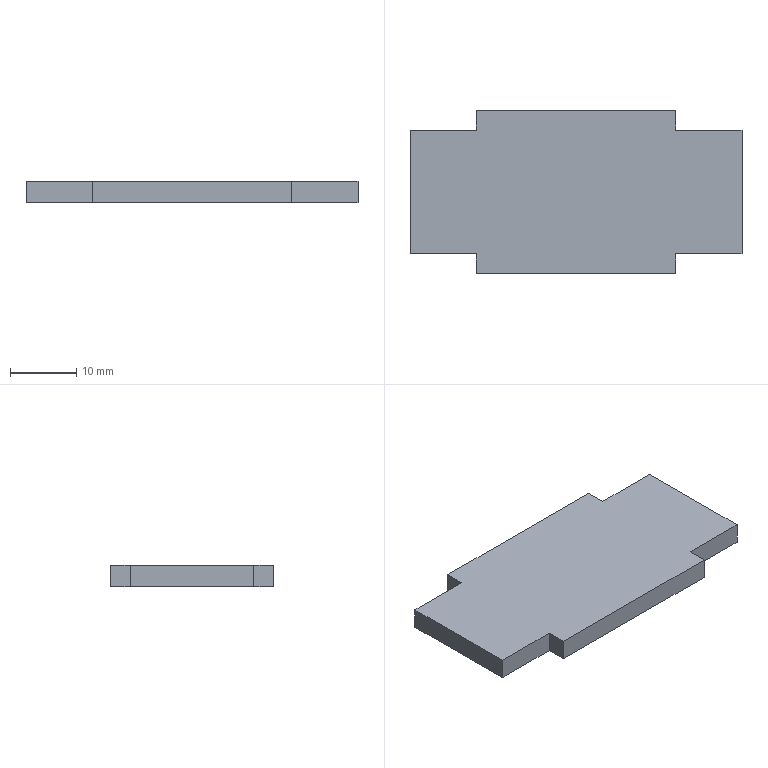Part | SolidWorks | features FlatPattern 1, SMBaseFlange 1, SheetMetal 1 | 1 solid | 14 faces | box 50 x 24.6 x 3.2 mm | volume 3552 mm3 | plane 14
STEP:
#1=CARTESIAN_POINT('',(95.,21.8,0.));
#2=VERTEX_POINT('',#1);
#3=CARTESIAN_POINT('',(95.,3.2,0.));
#4=VERTEX_POINT('',#3);
#5=CARTESIAN_POINT('',(95.,3.2,0.));
#6=DIRECTION('',(0.,-1.,0.));
#7=VECTOR('',#6,1000.);
#8=LINE('',#5,#7);
#9=EDGE_CURVE('',#2,#4,#8,.T.);
#10=ORIENTED_EDGE('',*,*,#9,.F.);
#11=CARTESIAN_POINT('',(95.,21.8,-3.2));
#12=VERTEX_POINT('',#11);
#13=CARTESIAN_POINT('',(95.,21.8,-3.2));
#14=DIRECTION('',(0.,0.,1.));
#15=VECTOR('',#14,1000.);
#16=LINE('',#13,#15);
#17=EDGE_CURVE('',#12,#2,#16,.T.);
#18=ORIENTED_EDGE('',*,*,#17,.F.);
#19=CARTESIAN_POINT('',(95.,3.2,-3.2));
#20=VERTEX_POINT('',#19);
#21=CARTESIAN_POINT('',(95.,3.2,-3.2));
#22=DIRECTION('',(0.,-1.,0.));
#23=VECTOR('',#22,1000.);
#24=LINE('',#21,#23);
#25=EDGE_CURVE('',#12,#20,#24,.T.);
#26=ORIENTED_EDGE('',*,*,#25,.T.);
#27=CARTESIAN_POINT('',(95.,3.2,-3.2));
#28=DIRECTION('',(0.,0.,1.));
#29=VECTOR('',#28,1000.);
#30=LINE('',#27,#29);
#31=EDGE_CURVE('',#20,#4,#30,.T.);
#32=ORIENTED_EDGE('',*,*,#31,.T.);
#33=EDGE_LOOP('',(#10,#18,#26,#32));
#34=FACE_OUTER_BOUND('',#33,.T.);
#35=CARTESIAN_POINT('',(95.,3.2,-3.2));
#36=DIRECTION('',(-1.,0.,0.));
#37=DIRECTION('',(0.,0.,1.));
#38=AXIS2_PLACEMENT_3D('',#35,#36,#37);
#39=PLANE('',#38);
#40=ADVANCED_FACE('',(#34),#39,.T.);
#41=CARTESIAN_POINT('',(105.,21.8,0.));
#42=VERTEX_POINT('',#41);
#43=CARTESIAN_POINT('',(95.,21.8,0.));
#44=DIRECTION('',(-1.,0.,0.));
#45=VECTOR('',#44,1000.);
#46=LINE('',#43,#45);
#47=EDGE_CURVE('',#42,#2,#46,.T.);
#48=ORIENTED_EDGE('',*,*,#47,.F.);
#49=CARTESIAN_POINT('',(105.,21.8,-3.2));
#50=VERTEX_POINT('',#49);
#51=CARTESIAN_POINT('',(105.,21.8,-3.2));
#52=DIRECTION('',(0.,0.,1.));
#53=VECTOR('',#52,1000.);
#54=LINE('',#51,#53);
#55=EDGE_CURVE('',#50,#42,#54,.T.);
#56=ORIENTED_EDGE('',*,*,#55,.F.);
#57=CARTESIAN_POINT('',(95.,21.8,-3.2));
#58=DIRECTION('',(-1.,0.,0.));
#59=VECTOR('',#58,1000.);
#60=LINE('',#57,#59);
#61=EDGE_CURVE('',#50,#12,#60,.T.);
#62=ORIENTED_EDGE('',*,*,#61,.T.);
#63=ORIENTED_EDGE('',*,*,#17,.T.);
#64=EDGE_LOOP('',(#48,#56,#62,#63));
#65=FACE_OUTER_BOUND('',#64,.T.);
#66=CARTESIAN_POINT('',(95.,21.8,-3.2));
#67=DIRECTION('',(0.,1.,0.));
#68=DIRECTION('',(0.,0.,1.));
#69=AXIS2_PLACEMENT_3D('',#66,#67,#68);
#70=PLANE('',#69);
#71=ADVANCED_FACE('',(#65),#70,.T.);
#72=CARTESIAN_POINT('',(105.,24.8,0.));
#73=VERTEX_POINT('',#72);
#74=CARTESIAN_POINT('',(105.,21.8,0.));
#75=DIRECTION('',(0.,-1.,0.));
#76=VECTOR('',#75,1000.);
#77=LINE('',#74,#76);
#78=EDGE_CURVE('',#73,#42,#77,.T.);
#79=ORIENTED_EDGE('',*,*,#78,.F.);
#80=CARTESIAN_POINT('',(105.,24.8,-3.2));
#81=VERTEX_POINT('',#80);
#82=CARTESIAN_POINT('',(105.,24.8,-3.2));
#83=DIRECTION('',(0.,0.,1.));
#84=VECTOR('',#83,1000.);
#85=LINE('',#82,#84);
#86=EDGE_CURVE('',#81,#73,#85,.T.);
#87=ORIENTED_EDGE('',*,*,#86,.F.);
#88=CARTESIAN_POINT('',(105.,21.8,-3.2));
#89=DIRECTION('',(0.,-1.,0.));
#90=VECTOR('',#89,1000.);
#91=LINE('',#88,#90);
#92=EDGE_CURVE('',#81,#50,#91,.T.);
#93=ORIENTED_EDGE('',*,*,#92,.T.);
#94=ORIENTED_EDGE('',*,*,#55,.T.);
#95=EDGE_LOOP('',(#79,#87,#93,#94));
#96=FACE_OUTER_BOUND('',#95,.T.);
#97=CARTESIAN_POINT('',(105.,21.8,-3.2));
#98=DIRECTION('',(-1.,0.,0.));
#99=DIRECTION('',(0.,0.,1.));
#100=AXIS2_PLACEMENT_3D('',#97,#98,#99);
#101=PLANE('',#100);
#102=ADVANCED_FACE('',(#96),#101,.T.);
#103=CARTESIAN_POINT('',(135.,24.8,0.));
#104=VERTEX_POINT('',#103);
#105=CARTESIAN_POINT('',(105.,24.8,0.));
#106=DIRECTION('',(-1.,0.,0.));
#107=VECTOR('',#106,1000.);
#108=LINE('',#105,#107);
#109=EDGE_CURVE('',#104,#73,#108,.T.);
#110=ORIENTED_EDGE('',*,*,#109,.F.);
#111=CARTESIAN_POINT('',(135.,24.8,-3.2));
#112=VERTEX_POINT('',#111);
#113=CARTESIAN_POINT('',(135.,24.8,-3.2));
#114=DIRECTION('',(0.,0.,1.));
#115=VECTOR('',#114,1000.);
#116=LINE('',#113,#115);
#117=EDGE_CURVE('',#112,#104,#116,.T.);
#118=ORIENTED_EDGE('',*,*,#117,.F.);
#119=CARTESIAN_POINT('',(105.,24.8,-3.2));
#120=DIRECTION('',(-1.,0.,0.));
#121=VECTOR('',#120,1000.);
#122=LINE('',#119,#121);
#123=EDGE_CURVE('',#112,#81,#122,.T.);
#124=ORIENTED_EDGE('',*,*,#123,.T.);
#125=ORIENTED_EDGE('',*,*,#86,.T.);
#126=EDGE_LOOP('',(#110,#118,#124,#125));
#127=FACE_OUTER_BOUND('',#126,.T.);
#128=CARTESIAN_POINT('',(105.,24.8,-3.2));
#129=DIRECTION('',(0.,1.,0.));
#130=DIRECTION('',(0.,0.,1.));
#131=AXIS2_PLACEMENT_3D('',#128,#129,#130);
#132=PLANE('',#131);
#133=ADVANCED_FACE('',(#127),#132,.T.);
#134=CARTESIAN_POINT('',(135.,21.8,0.));
#135=VERTEX_POINT('',#134);
#136=CARTESIAN_POINT('',(135.,24.8,0.));
#137=DIRECTION('',(0.,1.,0.));
#138=VECTOR('',#137,1000.);
#139=LINE('',#136,#138);
#140=EDGE_CURVE('',#135,#104,#139,.T.);
#141=ORIENTED_EDGE('',*,*,#140,.F.);
#142=CARTESIAN_POINT('',(135.,21.8,-3.2));
#143=VERTEX_POINT('',#142);
#144=CARTESIAN_POINT('',(135.,21.8,-3.2));
#145=DIRECTION('',(0.,0.,1.));
#146=VECTOR('',#145,1000.);
#147=LINE('',#144,#146);
#148=EDGE_CURVE('',#143,#135,#147,.T.);
#149=ORIENTED_EDGE('',*,*,#148,.F.);
#150=CARTESIAN_POINT('',(135.,24.8,-3.2));
#151=DIRECTION('',(0.,1.,0.));
#152=VECTOR('',#151,1000.);
#153=LINE('',#150,#152);
#154=EDGE_CURVE('',#143,#112,#153,.T.);
#155=ORIENTED_EDGE('',*,*,#154,.T.);
#156=ORIENTED_EDGE('',*,*,#117,.T.);
#157=EDGE_LOOP('',(#141,#149,#155,#156));
#158=FACE_OUTER_BOUND('',#157,.T.);
#159=CARTESIAN_POINT('',(135.,24.8,-3.2));
#160=DIRECTION('',(1.,0.,0.));
#161=DIRECTION('',(0.,0.,-1.));
#162=AXIS2_PLACEMENT_3D('',#159,#160,#161);
#163=PLANE('',#162);
#164=ADVANCED_FACE('',(#158),#163,.T.);
#165=CARTESIAN_POINT('',(145.,21.8,0.));
#166=VERTEX_POINT('',#165);
#167=CARTESIAN_POINT('',(135.,21.8,0.));
#168=DIRECTION('',(-1.,0.,0.));
#169=VECTOR('',#168,1000.);
#170=LINE('',#167,#169);
#171=EDGE_CURVE('',#166,#135,#170,.T.);
#172=ORIENTED_EDGE('',*,*,#171,.F.);
#173=CARTESIAN_POINT('',(145.,21.8,-3.2));
#174=VERTEX_POINT('',#173);
#175=CARTESIAN_POINT('',(145.,21.8,-3.2));
#176=DIRECTION('',(0.,0.,1.));
#177=VECTOR('',#176,1000.);
#178=LINE('',#175,#177);
#179=EDGE_CURVE('',#174,#166,#178,.T.);
#180=ORIENTED_EDGE('',*,*,#179,.F.);
#181=CARTESIAN_POINT('',(135.,21.8,-3.2));
#182=DIRECTION('',(-1.,0.,0.));
#183=VECTOR('',#182,1000.);
#184=LINE('',#181,#183);
#185=EDGE_CURVE('',#174,#143,#184,.T.);
#186=ORIENTED_EDGE('',*,*,#185,.T.);
#187=ORIENTED_EDGE('',*,*,#148,.T.);
#188=EDGE_LOOP('',(#172,#180,#186,#187));
#189=FACE_OUTER_BOUND('',#188,.T.);
#190=CARTESIAN_POINT('',(135.,21.8,-3.2));
#191=DIRECTION('',(0.,1.,0.));
#192=DIRECTION('',(0.,0.,1.));
#193=AXIS2_PLACEMENT_3D('',#190,#191,#192);
#194=PLANE('',#193);
#195=ADVANCED_FACE('',(#189),#194,.T.);
#196=CARTESIAN_POINT('',(145.,3.2,0.));
#197=VERTEX_POINT('',#196);
#198=CARTESIAN_POINT('',(145.,3.2,0.));
#199=DIRECTION('',(0.,1.,0.));
#200=VECTOR('',#199,1000.);
#201=LINE('',#198,#200);
#202=EDGE_CURVE('',#197,#166,#201,.T.);
#203=ORIENTED_EDGE('',*,*,#202,.F.);
#204=CARTESIAN_POINT('',(145.,3.2,-3.2));
#205=VERTEX_POINT('',#204);
#206=CARTESIAN_POINT('',(145.,3.2,-3.2));
#207=DIRECTION('',(0.,0.,1.));
#208=VECTOR('',#207,1000.);
#209=LINE('',#206,#208);
#210=EDGE_CURVE('',#205,#197,#209,.T.);
#211=ORIENTED_EDGE('',*,*,#210,.F.);
#212=CARTESIAN_POINT('',(145.,3.2,-3.2));
#213=DIRECTION('',(0.,1.,0.));
#214=VECTOR('',#213,1000.);
#215=LINE('',#212,#214);
#216=EDGE_CURVE('',#205,#174,#215,.T.);
#217=ORIENTED_EDGE('',*,*,#216,.T.);
#218=ORIENTED_EDGE('',*,*,#179,.T.);
#219=EDGE_LOOP('',(#203,#211,#217,#218));
#220=FACE_OUTER_BOUND('',#219,.T.);
#221=CARTESIAN_POINT('',(145.,3.2,-3.2));
#222=DIRECTION('',(1.,0.,0.));
#223=DIRECTION('',(0.,0.,-1.));
#224=AXIS2_PLACEMENT_3D('',#221,#222,#223);
#225=PLANE('',#224);
#226=ADVANCED_FACE('',(#220),#225,.T.);
#227=CARTESIAN_POINT('',(135.,3.2,0.));
#228=VERTEX_POINT('',#227);
#229=CARTESIAN_POINT('',(135.,3.2,0.));
#230=DIRECTION('',(1.,0.,0.));
#231=VECTOR('',#230,1000.);
#232=LINE('',#229,#231);
#233=EDGE_CURVE('',#228,#197,#232,.T.);
#234=ORIENTED_EDGE('',*,*,#233,.F.);
#235=CARTESIAN_POINT('',(135.,3.2,-3.2));
#236=VERTEX_POINT('',#235);
#237=CARTESIAN_POINT('',(135.,3.2,-3.2));
#238=DIRECTION('',(0.,0.,1.));
#239=VECTOR('',#238,1000.);
#240=LINE('',#237,#239);
#241=EDGE_CURVE('',#236,#228,#240,.T.);
#242=ORIENTED_EDGE('',*,*,#241,.F.);
#243=CARTESIAN_POINT('',(135.,3.2,-3.2));
#244=DIRECTION('',(1.,0.,0.));
#245=VECTOR('',#244,1000.);
#246=LINE('',#243,#245);
#247=EDGE_CURVE('',#236,#205,#246,.T.);
#248=ORIENTED_EDGE('',*,*,#247,.T.);
#249=ORIENTED_EDGE('',*,*,#210,.T.);
#250=EDGE_LOOP('',(#234,#242,#248,#249));
#251=FACE_OUTER_BOUND('',#250,.T.);
#252=CARTESIAN_POINT('',(135.,3.2,-3.2));
#253=DIRECTION('',(0.,-1.,0.));
#254=DIRECTION('',(0.,0.,-1.));
#255=AXIS2_PLACEMENT_3D('',#252,#253,#254);
#256=PLANE('',#255);
#257=ADVANCED_FACE('',(#251),#256,.T.);
#258=CARTESIAN_POINT('',(135.,0.2,0.));
#259=VERTEX_POINT('',#258);
#260=CARTESIAN_POINT('',(135.,0.2,0.));
#261=DIRECTION('',(0.,1.,0.));
#262=VECTOR('',#261,1000.);
#263=LINE('',#260,#262);
#264=EDGE_CURVE('',#259,#228,#263,.T.);
#265=ORIENTED_EDGE('',*,*,#264,.F.);
#266=CARTESIAN_POINT('',(135.,0.2,-3.2));
#267=VERTEX_POINT('',#266);
#268=CARTESIAN_POINT('',(135.,0.2,-3.2));
#269=DIRECTION('',(0.,0.,1.));
#270=VECTOR('',#269,1000.);
#271=LINE('',#268,#270);
#272=EDGE_CURVE('',#267,#259,#271,.T.);
#273=ORIENTED_EDGE('',*,*,#272,.F.);
#274=CARTESIAN_POINT('',(135.,0.2,-3.2));
#275=DIRECTION('',(0.,1.,0.));
#276=VECTOR('',#275,1000.);
#277=LINE('',#274,#276);
#278=EDGE_CURVE('',#267,#236,#277,.T.);
#279=ORIENTED_EDGE('',*,*,#278,.T.);
#280=ORIENTED_EDGE('',*,*,#241,.T.);
#281=EDGE_LOOP('',(#265,#273,#279,#280));
#282=FACE_OUTER_BOUND('',#281,.T.);
#283=CARTESIAN_POINT('',(135.,0.2,-3.2));
#284=DIRECTION('',(1.,0.,0.));
#285=DIRECTION('',(0.,0.,-1.));
#286=AXIS2_PLACEMENT_3D('',#283,#284,#285);
#287=PLANE('',#286);
#288=ADVANCED_FACE('',(#282),#287,.T.);
#289=CARTESIAN_POINT('',(105.,0.2,0.));
#290=VERTEX_POINT('',#289);
#291=CARTESIAN_POINT('',(105.,0.2,0.));
#292=DIRECTION('',(1.,0.,0.));
#293=VECTOR('',#292,1000.);
#294=LINE('',#291,#293);
#295=EDGE_CURVE('',#290,#259,#294,.T.);
#296=ORIENTED_EDGE('',*,*,#295,.F.);
#297=CARTESIAN_POINT('',(105.,0.2,-3.2));
#298=VERTEX_POINT('',#297);
#299=CARTESIAN_POINT('',(105.,0.2,-3.2));
#300=DIRECTION('',(0.,0.,1.));
#301=VECTOR('',#300,1000.);
#302=LINE('',#299,#301);
#303=EDGE_CURVE('',#298,#290,#302,.T.);
#304=ORIENTED_EDGE('',*,*,#303,.F.);
#305=CARTESIAN_POINT('',(105.,0.2,-3.2));
#306=DIRECTION('',(1.,0.,0.));
#307=VECTOR('',#306,1000.);
#308=LINE('',#305,#307);
#309=EDGE_CURVE('',#298,#267,#308,.T.);
#310=ORIENTED_EDGE('',*,*,#309,.T.);
#311=ORIENTED_EDGE('',*,*,#272,.T.);
#312=EDGE_LOOP('',(#296,#304,#310,#311));
#313=FACE_OUTER_BOUND('',#312,.T.);
#314=CARTESIAN_POINT('',(105.,0.2,-3.2));
#315=DIRECTION('',(0.,-1.,0.));
#316=DIRECTION('',(0.,0.,-1.));
#317=AXIS2_PLACEMENT_3D('',#314,#315,#316);
#318=PLANE('',#317);
#319=ADVANCED_FACE('',(#313),#318,.T.);
#320=CARTESIAN_POINT('',(105.,3.2,0.));
#321=VERTEX_POINT('',#320);
#322=CARTESIAN_POINT('',(105.,3.2,0.));
#323=DIRECTION('',(0.,-1.,0.));
#324=VECTOR('',#323,1000.);
#325=LINE('',#322,#324);
#326=EDGE_CURVE('',#321,#290,#325,.T.);
#327=ORIENTED_EDGE('',*,*,#326,.F.);
#328=CARTESIAN_POINT('',(105.,3.2,-3.2));
#329=VERTEX_POINT('',#328);
#330=CARTESIAN_POINT('',(105.,3.2,-3.2));
#331=DIRECTION('',(0.,0.,1.));
#332=VECTOR('',#331,1000.);
#333=LINE('',#330,#332);
#334=EDGE_CURVE('',#329,#321,#333,.T.);
#335=ORIENTED_EDGE('',*,*,#334,.F.);
#336=CARTESIAN_POINT('',(105.,3.2,-3.2));
#337=DIRECTION('',(0.,-1.,0.));
#338=VECTOR('',#337,1000.);
#339=LINE('',#336,#338);
#340=EDGE_CURVE('',#329,#298,#339,.T.);
#341=ORIENTED_EDGE('',*,*,#340,.T.);
#342=ORIENTED_EDGE('',*,*,#303,.T.);
#343=EDGE_LOOP('',(#327,#335,#341,#342));
#344=FACE_OUTER_BOUND('',#343,.T.);
#345=CARTESIAN_POINT('',(105.,3.2,-3.2));
#346=DIRECTION('',(-1.,0.,0.));
#347=DIRECTION('',(0.,0.,1.));
#348=AXIS2_PLACEMENT_3D('',#345,#346,#347);
#349=PLANE('',#348);
#350=ADVANCED_FACE('',(#344),#349,.T.);
#351=CARTESIAN_POINT('',(95.,3.2,0.));
#352=DIRECTION('',(1.,0.,0.));
#353=VECTOR('',#352,1000.);
#354=LINE('',#351,#353);
#355=EDGE_CURVE('',#4,#321,#354,.T.);
#356=ORIENTED_EDGE('',*,*,#355,.F.);
#357=ORIENTED_EDGE('',*,*,#31,.F.);
#358=CARTESIAN_POINT('',(95.,3.2,-3.2));
#359=DIRECTION('',(1.,0.,0.));
#360=VECTOR('',#359,1000.);
#361=LINE('',#358,#360);
#362=EDGE_CURVE('',#20,#329,#361,.T.);
#363=ORIENTED_EDGE('',*,*,#362,.T.);
#364=ORIENTED_EDGE('',*,*,#334,.T.);
#365=EDGE_LOOP('',(#356,#357,#363,#364));
#366=FACE_OUTER_BOUND('',#365,.T.);
#367=CARTESIAN_POINT('',(95.,3.2,-3.2));
#368=DIRECTION('',(0.,-1.,0.));
#369=DIRECTION('',(0.,0.,-1.));
#370=AXIS2_PLACEMENT_3D('',#367,#368,#369);
#371=PLANE('',#370);
#372=ADVANCED_FACE('',(#366),#371,.T.);
#373=ORIENTED_EDGE('',*,*,#25,.F.);
#374=ORIENTED_EDGE('',*,*,#61,.F.);
#375=ORIENTED_EDGE('',*,*,#92,.F.);
#376=ORIENTED_EDGE('',*,*,#123,.F.);
#377=ORIENTED_EDGE('',*,*,#154,.F.);
#378=ORIENTED_EDGE('',*,*,#185,.F.);
#379=ORIENTED_EDGE('',*,*,#216,.F.);
#380=ORIENTED_EDGE('',*,*,#247,.F.);
#381=ORIENTED_EDGE('',*,*,#278,.F.);
#382=ORIENTED_EDGE('',*,*,#309,.F.);
#383=ORIENTED_EDGE('',*,*,#340,.F.);
#384=ORIENTED_EDGE('',*,*,#362,.F.);
#385=EDGE_LOOP('',(#373,#374,#375,#376,#377,#378,#379,#380,#381,#382,#383,#384));
#386=FACE_OUTER_BOUND('',#385,.T.);
#387=CARTESIAN_POINT('',(0.,0.,-3.2));
#388=DIRECTION('',(0.,0.,-1.));
#389=DIRECTION('',(-1.,0.,0.));
#390=AXIS2_PLACEMENT_3D('',#387,#388,#389);
#391=PLANE('',#390);
#392=ADVANCED_FACE('',(#386),#391,.T.);
#393=ORIENTED_EDGE('',*,*,#9,.T.);
#394=ORIENTED_EDGE('',*,*,#355,.T.);
#395=ORIENTED_EDGE('',*,*,#326,.T.);
#396=ORIENTED_EDGE('',*,*,#295,.T.);
#397=ORIENTED_EDGE('',*,*,#264,.T.);
#398=ORIENTED_EDGE('',*,*,#233,.T.);
#399=ORIENTED_EDGE('',*,*,#202,.T.);
#400=ORIENTED_EDGE('',*,*,#171,.T.);
#401=ORIENTED_EDGE('',*,*,#140,.T.);
#402=ORIENTED_EDGE('',*,*,#109,.T.);
#403=ORIENTED_EDGE('',*,*,#78,.T.);
#404=ORIENTED_EDGE('',*,*,#47,.T.);
#405=EDGE_LOOP('',(#393,#394,#395,#396,#397,#398,#399,#400,#401,#402,#403,#404));
#406=FACE_OUTER_BOUND('',#405,.T.);
#407=CARTESIAN_POINT('',(0.,0.,0.));
#408=DIRECTION('',(0.,0.,-1.));
#409=DIRECTION('',(-1.,0.,0.));
#410=AXIS2_PLACEMENT_3D('',#407,#408,#409);
#411=PLANE('',#410);
#412=ADVANCED_FACE('',(#406),#411,.F.);
#413=CLOSED_SHELL('',(#40,#71,#102,#133,#164,#195,#226,#257,#288,#319,#350,#372,#392,#412));
#414=MANIFOLD_SOLID_BREP('',#413);
#415=CARTESIAN_POINT('',(0.,0.,0.));
#416=DIRECTION('',(0.,0.,1.));
#417=DIRECTION('',(1.,0.,0.));
#418=AXIS2_PLACEMENT_3D('',#415,#416,#417);
#419=(LENGTH_UNIT()NAMED_UNIT(*)SI_UNIT(.MILLI.,.METRE.));
#420=UNCERTAINTY_MEASURE_WITH_UNIT(LENGTH_MEASURE(0.00001),#419,'','');
#421=(NAMED_UNIT(*)PLANE_ANGLE_UNIT()SI_UNIT($,.RADIAN.));
#422=(NAMED_UNIT(*)SI_UNIT($,.STERADIAN.)SOLID_ANGLE_UNIT());
#423=(GEOMETRIC_REPRESENTATION_CONTEXT(3)GLOBAL_UNCERTAINTY_ASSIGNED_CONTEXT((#420))GLOBAL_UNIT_ASSIGNED_CONTEXT((#419,#421,#422))REPRESENTATION_CONTEXT('',''));
#424=ADVANCED_BREP_SHAPE_REPRESENTATION('',(#414,#418),#423);